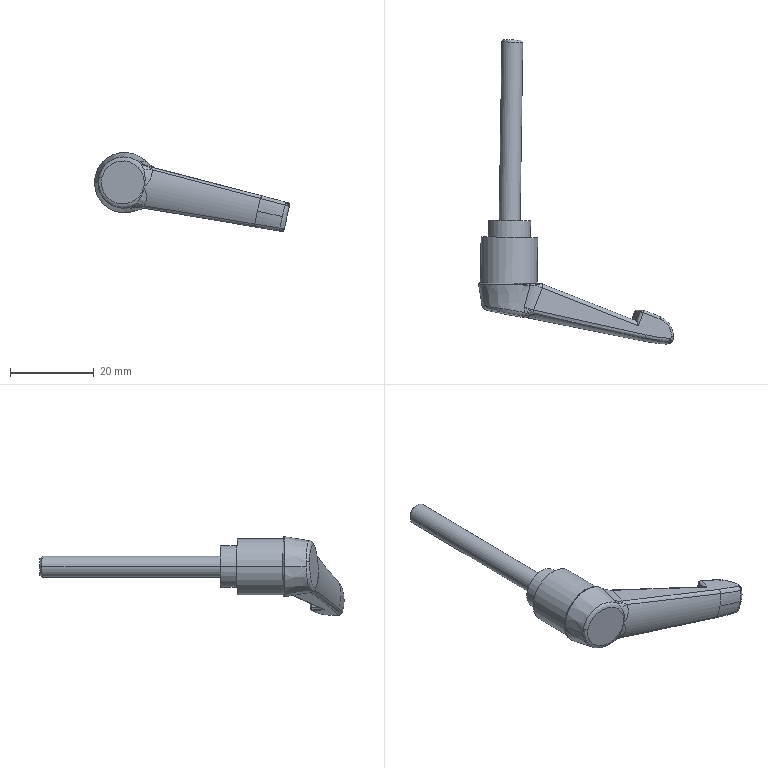Part | SolidWorks | features BaseBody 1 | 1 solid | 76 faces | box 46.508 x 72.59 x 18.825 mm | volume 5501 mm3 | spline 43 | cylinder 18 | plane 11 | cone 4 | commonest cylinder face diameters 1.2 x6 10 x3 2 x2 5 x2 13.5 x2 0.4 x1